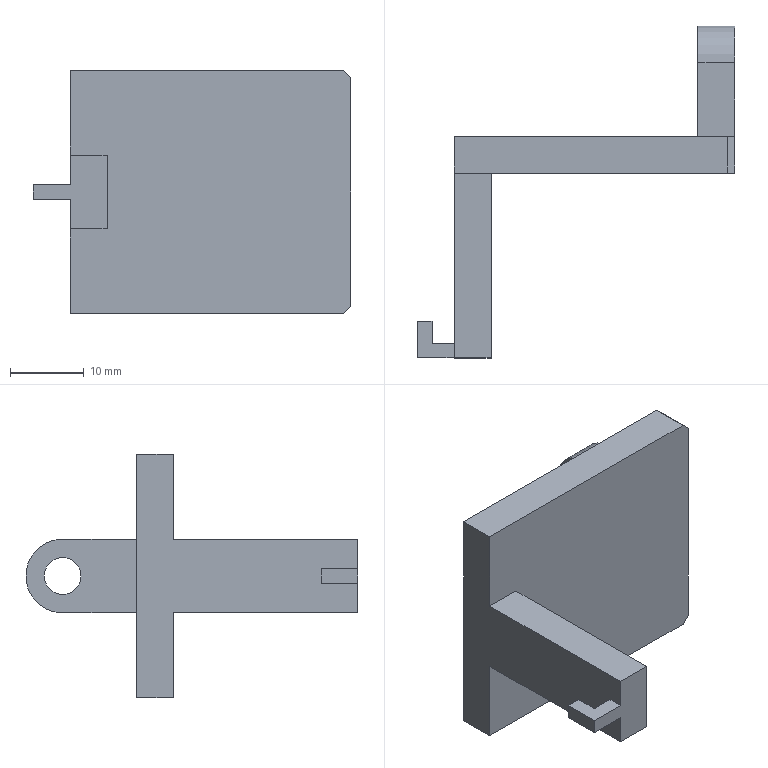Part | SolidWorks | 1 solid | 24 faces | box 43 x 45 x 33 mm | volume 8145 mm3 | plane 21 | cylinder 3 | commonest cylinder face diameters 5 x2 10 x1
STEP:
#1=CARTESIAN_POINT('',(30.5,25.,2.5));
#2=VERTEX_POINT('',#1);
#3=CARTESIAN_POINT('',(30.5,25.,-2.5));
#4=VERTEX_POINT('',#3);
#5=CARTESIAN_POINT('',(30.5,25.,0.));
#6=DIRECTION('',(1.,0.,0.));
#7=DIRECTION('',(0.,0.,-1.));
#8=AXIS2_PLACEMENT_3D('',#5,#6,#7);
#9=CIRCLE('',#8,2.5);
#10=EDGE_CURVE('',#2,#4,#9,.T.);
#11=ORIENTED_EDGE('',*,*,#10,.F.);
#12=CARTESIAN_POINT('',(35.5,25.,2.5));
#13=VERTEX_POINT('',#12);
#14=CARTESIAN_POINT('',(5.5,25.,2.5));
#15=DIRECTION('',(1.,0.,0.));
#16=VECTOR('',#15,1000.);
#17=LINE('',#14,#16);
#18=EDGE_CURVE('',#2,#13,#17,.T.);
#19=ORIENTED_EDGE('',*,*,#18,.T.);
#20=CARTESIAN_POINT('',(35.5,25.,-2.5));
#21=VERTEX_POINT('',#20);
#22=CARTESIAN_POINT('',(35.5,25.,0.));
#23=DIRECTION('',(1.,0.,0.));
#24=DIRECTION('',(0.,0.,-1.));
#25=AXIS2_PLACEMENT_3D('',#22,#23,#24);
#26=CIRCLE('',#25,2.5);
#27=EDGE_CURVE('',#13,#21,#26,.T.);
#28=ORIENTED_EDGE('',*,*,#27,.T.);
#29=CARTESIAN_POINT('',(5.5,25.,-2.5));
#30=DIRECTION('',(1.,0.,0.));
#31=VECTOR('',#30,1000.);
#32=LINE('',#29,#31);
#33=EDGE_CURVE('',#4,#21,#32,.T.);
#34=ORIENTED_EDGE('',*,*,#33,.F.);
#35=EDGE_LOOP('',(#11,#19,#28,#34));
#36=FACE_OUTER_BOUND('',#35,.T.);
#37=CARTESIAN_POINT('',(5.5,25.,0.));
#38=DIRECTION('',(1.,0.,0.));
#39=DIRECTION('',(0.,0.,-1.));
#40=AXIS2_PLACEMENT_3D('',#37,#38,#39);
#41=CYLINDRICAL_SURFACE('',#40,2.5);
#42=ADVANCED_FACE('',(#36),#41,.F.);
#43=CARTESIAN_POINT('',(-2.5,-13.,-1.));
#44=VERTEX_POINT('',#43);
#45=CARTESIAN_POINT('',(-2.5,-15.,-1.));
#46=VERTEX_POINT('',#45);
#47=CARTESIAN_POINT('',(-2.5,-15.,-1.));
#48=DIRECTION('',(0.,-1.,0.));
#49=VECTOR('',#48,1000.);
#50=LINE('',#47,#49);
#51=EDGE_CURVE('',#44,#46,#50,.T.);
#52=ORIENTED_EDGE('',*,*,#51,.F.);
#53=CARTESIAN_POINT('',(-2.5,-13.,1.));
#54=VERTEX_POINT('',#53);
#55=CARTESIAN_POINT('',(-2.5,-13.,1.));
#56=DIRECTION('',(0.,0.,-1.));
#57=VECTOR('',#56,1000.);
#58=LINE('',#55,#57);
#59=EDGE_CURVE('',#54,#44,#58,.T.);
#60=ORIENTED_EDGE('',*,*,#59,.F.);
#61=CARTESIAN_POINT('',(-2.5,-15.,1.));
#62=VERTEX_POINT('',#61);
#63=CARTESIAN_POINT('',(-2.5,-15.,1.));
#64=DIRECTION('',(0.,-1.,0.));
#65=VECTOR('',#64,1000.);
#66=LINE('',#63,#65);
#67=EDGE_CURVE('',#54,#62,#66,.T.);
#68=ORIENTED_EDGE('',*,*,#67,.T.);
#69=CARTESIAN_POINT('',(-2.5,-15.,5.));
#70=VERTEX_POINT('',#69);
#71=CARTESIAN_POINT('',(-2.5,-15.,16.5));
#72=DIRECTION('',(0.,0.,-1.));
#73=VECTOR('',#72,1000.);
#74=LINE('',#71,#73);
#75=EDGE_CURVE('',#70,#62,#74,.T.);
#76=ORIENTED_EDGE('',*,*,#75,.F.);
#77=CARTESIAN_POINT('',(-2.5,10.,5.));
#78=VERTEX_POINT('',#77);
#79=CARTESIAN_POINT('',(-2.5,0.,5.));
#80=DIRECTION('',(0.,1.,0.));
#81=VECTOR('',#80,1000.);
#82=LINE('',#79,#81);
#83=EDGE_CURVE('',#70,#78,#82,.T.);
#84=ORIENTED_EDGE('',*,*,#83,.T.);
#85=CARTESIAN_POINT('',(-2.5,10.,16.5));
#86=VERTEX_POINT('',#85);
#87=CARTESIAN_POINT('',(-2.5,10.,16.5));
#88=DIRECTION('',(0.,0.,1.));
#89=VECTOR('',#88,1000.);
#90=LINE('',#87,#89);
#91=EDGE_CURVE('',#78,#86,#90,.T.);
#92=ORIENTED_EDGE('',*,*,#91,.T.);
#93=CARTESIAN_POINT('',(-2.5,15.,16.5));
#94=VERTEX_POINT('',#93);
#95=CARTESIAN_POINT('',(-2.5,0.,16.5));
#96=DIRECTION('',(0.,-1.,0.));
#97=VECTOR('',#96,1000.);
#98=LINE('',#95,#97);
#99=EDGE_CURVE('',#94,#86,#98,.T.);
#100=ORIENTED_EDGE('',*,*,#99,.F.);
#101=CARTESIAN_POINT('',(-2.5,15.,-16.5));
#102=VERTEX_POINT('',#101);
#103=CARTESIAN_POINT('',(-2.5,15.,16.5));
#104=DIRECTION('',(0.,0.,-1.));
#105=VECTOR('',#104,1000.);
#106=LINE('',#103,#105);
#107=EDGE_CURVE('',#94,#102,#106,.T.);
#108=ORIENTED_EDGE('',*,*,#107,.T.);
#109=CARTESIAN_POINT('',(-2.5,10.,-16.5));
#110=VERTEX_POINT('',#109);
#111=CARTESIAN_POINT('',(-2.5,0.,-16.5));
#112=DIRECTION('',(0.,-1.,0.));
#113=VECTOR('',#112,1000.);
#114=LINE('',#111,#113);
#115=EDGE_CURVE('',#102,#110,#114,.T.);
#116=ORIENTED_EDGE('',*,*,#115,.T.);
#117=CARTESIAN_POINT('',(-2.5,10.,-5.));
#118=VERTEX_POINT('',#117);
#119=CARTESIAN_POINT('',(-2.5,10.,16.5));
#120=DIRECTION('',(0.,0.,1.));
#121=VECTOR('',#120,1000.);
#122=LINE('',#119,#121);
#123=EDGE_CURVE('',#110,#118,#122,.T.);
#124=ORIENTED_EDGE('',*,*,#123,.T.);
#125=CARTESIAN_POINT('',(-2.5,-15.,-5.));
#126=VERTEX_POINT('',#125);
#127=CARTESIAN_POINT('',(-2.5,0.,-5.));
#128=DIRECTION('',(0.,-1.,0.));
#129=VECTOR('',#128,1000.);
#130=LINE('',#127,#129);
#131=EDGE_CURVE('',#118,#126,#130,.T.);
#132=ORIENTED_EDGE('',*,*,#131,.T.);
#133=CARTESIAN_POINT('',(-2.5,-15.,16.5));
#134=DIRECTION('',(0.,0.,-1.));
#135=VECTOR('',#134,1000.);
#136=LINE('',#133,#135);
#137=EDGE_CURVE('',#46,#126,#136,.T.);
#138=ORIENTED_EDGE('',*,*,#137,.F.);
#139=EDGE_LOOP('',(#52,#60,#68,#76,#84,#92,#100,#108,#116,#124,#132,#138));
#140=FACE_OUTER_BOUND('',#139,.T.);
#141=CARTESIAN_POINT('',(-2.5,0.,16.5));
#142=DIRECTION('',(1.,0.,0.));
#143=DIRECTION('',(0.,1.,0.));
#144=AXIS2_PLACEMENT_3D('',#141,#142,#143);
#145=PLANE('',#144);
#146=ADVANCED_FACE('',(#140),#145,.F.);
#147=CARTESIAN_POINT('',(35.5,25.,0.));
#148=DIRECTION('',(1.,0.,0.));
#149=DIRECTION('',(0.,0.,-1.));
#150=AXIS2_PLACEMENT_3D('',#147,#148,#149);
#151=CIRCLE('',#150,2.5);
#152=EDGE_CURVE('',#21,#13,#151,.T.);
#153=ORIENTED_EDGE('',*,*,#152,.F.);
#154=ORIENTED_EDGE('',*,*,#27,.F.);
#155=EDGE_LOOP('',(#153,#154));
#156=FACE_BOUND('',#155,.T.);
#157=CARTESIAN_POINT('',(35.5,10.,15.5));
#158=VERTEX_POINT('',#157);
#159=CARTESIAN_POINT('',(35.5,10.,-15.5));
#160=VERTEX_POINT('',#159);
#161=CARTESIAN_POINT('',(35.5,10.,16.5));
#162=DIRECTION('',(0.,0.,-1.));
#163=VECTOR('',#162,1000.);
#164=LINE('',#161,#163);
#165=EDGE_CURVE('',#158,#160,#164,.T.);
#166=ORIENTED_EDGE('',*,*,#165,.T.);
#167=CARTESIAN_POINT('',(35.5,15.,-15.5));
#168=VERTEX_POINT('',#167);
#169=CARTESIAN_POINT('',(35.5,15.,-15.5));
#170=DIRECTION('',(0.,1.,0.));
#171=VECTOR('',#170,1000.);
#172=LINE('',#169,#171);
#173=EDGE_CURVE('',#160,#168,#172,.T.);
#174=ORIENTED_EDGE('',*,*,#173,.T.);
#175=CARTESIAN_POINT('',(35.5,15.,-5.));
#176=VERTEX_POINT('',#175);
#177=CARTESIAN_POINT('',(35.5,15.,16.5));
#178=DIRECTION('',(0.,0.,-1.));
#179=VECTOR('',#178,1000.);
#180=LINE('',#177,#179);
#181=EDGE_CURVE('',#176,#168,#180,.T.);
#182=ORIENTED_EDGE('',*,*,#181,.F.);
#183=CARTESIAN_POINT('',(35.5,25.,-5.));
#184=VERTEX_POINT('',#183);
#185=CARTESIAN_POINT('',(35.5,0.,-5.));
#186=DIRECTION('',(0.,1.,0.));
#187=VECTOR('',#186,1000.);
#188=LINE('',#185,#187);
#189=EDGE_CURVE('',#176,#184,#188,.T.);
#190=ORIENTED_EDGE('',*,*,#189,.T.);
#191=CARTESIAN_POINT('',(35.5,25.,5.));
#192=VERTEX_POINT('',#191);
#193=CARTESIAN_POINT('',(35.5,25.,0.));
#194=DIRECTION('',(1.,0.,0.));
#195=DIRECTION('',(0.,0.,-1.));
#196=AXIS2_PLACEMENT_3D('',#193,#194,#195);
#197=CIRCLE('',#196,5.);
#198=EDGE_CURVE('',#184,#192,#197,.T.);
#199=ORIENTED_EDGE('',*,*,#198,.T.);
#200=CARTESIAN_POINT('',(35.5,15.,5.));
#201=VERTEX_POINT('',#200);
#202=CARTESIAN_POINT('',(35.5,0.,5.));
#203=DIRECTION('',(0.,1.,0.));
#204=VECTOR('',#203,1000.);
#205=LINE('',#202,#204);
#206=EDGE_CURVE('',#201,#192,#205,.T.);
#207=ORIENTED_EDGE('',*,*,#206,.F.);
#208=CARTESIAN_POINT('',(35.5,15.,15.5));
#209=VERTEX_POINT('',#208);
#210=CARTESIAN_POINT('',(35.5,15.,16.5));
#211=DIRECTION('',(0.,0.,-1.));
#212=VECTOR('',#211,1000.);
#213=LINE('',#210,#212);
#214=EDGE_CURVE('',#209,#201,#213,.T.);
#215=ORIENTED_EDGE('',*,*,#214,.F.);
#216=CARTESIAN_POINT('',(35.5,0.,15.5));
#217=DIRECTION('',(0.,-1.,0.));
#218=VECTOR('',#217,1000.);
#219=LINE('',#216,#218);
#220=EDGE_CURVE('',#209,#158,#219,.T.);
#221=ORIENTED_EDGE('',*,*,#220,.T.);
#222=EDGE_LOOP('',(#166,#174,#182,#190,#199,#207,#215,#221));
#223=FACE_OUTER_BOUND('',#222,.T.);
#224=CARTESIAN_POINT('',(35.5,0.,16.5));
#225=DIRECTION('',(1.,0.,0.));
#226=DIRECTION('',(0.,1.,0.));
#227=AXIS2_PLACEMENT_3D('',#224,#225,#226);
#228=PLANE('',#227);
#229=ADVANCED_FACE('',(#156,#223),#228,.T.);
#230=ORIENTED_EDGE('',*,*,#181,.T.);
#231=CARTESIAN_POINT('',(34.5,15.,-16.5));
#232=VERTEX_POINT('',#231);
#233=CARTESIAN_POINT('',(33.75,15.,-17.25));
#234=DIRECTION('',(-0.7071,0.,-0.7071));
#235=VECTOR('',#234,1000.);
#236=LINE('',#233,#235);
#237=EDGE_CURVE('',#168,#232,#236,.T.);
#238=ORIENTED_EDGE('',*,*,#237,.T.);
#239=CARTESIAN_POINT('',(0.,15.,-16.5));
#240=DIRECTION('',(1.,0.,0.));
#241=VECTOR('',#240,1000.);
#242=LINE('',#239,#241);
#243=EDGE_CURVE('',#102,#232,#242,.T.);
#244=ORIENTED_EDGE('',*,*,#243,.F.);
#245=ORIENTED_EDGE('',*,*,#107,.F.);
#246=CARTESIAN_POINT('',(34.5,15.,16.5));
#247=VERTEX_POINT('',#246);
#248=CARTESIAN_POINT('',(0.,15.,16.5));
#249=DIRECTION('',(1.,0.,0.));
#250=VECTOR('',#249,1000.);
#251=LINE('',#248,#250);
#252=EDGE_CURVE('',#94,#247,#251,.T.);
#253=ORIENTED_EDGE('',*,*,#252,.T.);
#254=CARTESIAN_POINT('',(17.25,15.,33.75));
#255=DIRECTION('',(0.7071,0.,-0.7071));
#256=VECTOR('',#255,1000.);
#257=LINE('',#254,#256);
#258=EDGE_CURVE('',#247,#209,#257,.T.);
#259=ORIENTED_EDGE('',*,*,#258,.T.);
#260=ORIENTED_EDGE('',*,*,#214,.T.);
#261=CARTESIAN_POINT('',(30.5,15.,5.));
#262=VERTEX_POINT('',#261);
#263=CARTESIAN_POINT('',(30.5,15.,5.));
#264=DIRECTION('',(1.,0.,0.));
#265=VECTOR('',#264,1000.);
#266=LINE('',#263,#265);
#267=EDGE_CURVE('',#262,#201,#266,.T.);
#268=ORIENTED_EDGE('',*,*,#267,.F.);
#269=CARTESIAN_POINT('',(30.5,15.,-5.));
#270=VERTEX_POINT('',#269);
#271=CARTESIAN_POINT('',(30.5,15.,0.));
#272=DIRECTION('',(0.,0.,1.));
#273=VECTOR('',#272,1000.);
#274=LINE('',#271,#273);
#275=EDGE_CURVE('',#270,#262,#274,.T.);
#276=ORIENTED_EDGE('',*,*,#275,.F.);
#277=CARTESIAN_POINT('',(30.5,15.,-5.));
#278=DIRECTION('',(1.,0.,0.));
#279=VECTOR('',#278,1000.);
#280=LINE('',#277,#279);
#281=EDGE_CURVE('',#270,#176,#280,.T.);
#282=ORIENTED_EDGE('',*,*,#281,.T.);
#283=EDGE_LOOP('',(#230,#238,#244,#245,#253,#259,#260,#268,#276,#282));
#284=FACE_OUTER_BOUND('',#283,.T.);
#285=CARTESIAN_POINT('',(0.,15.,16.5));
#286=DIRECTION('',(0.,1.,0.));
#287=DIRECTION('',(0.,0.,1.));
#288=AXIS2_PLACEMENT_3D('',#285,#286,#287);
#289=PLANE('',#288);
#290=ADVANCED_FACE('',(#284),#289,.T.);
#291=CARTESIAN_POINT('',(2.5,-15.,5.));
#292=VERTEX_POINT('',#291);
#293=CARTESIAN_POINT('',(2.5,-15.,-5.));
#294=VERTEX_POINT('',#293);
#295=CARTESIAN_POINT('',(2.5,-15.,16.5));
#296=DIRECTION('',(0.,0.,-1.));
#297=VECTOR('',#296,1000.);
#298=LINE('',#295,#297);
#299=EDGE_CURVE('',#292,#294,#298,.T.);
#300=ORIENTED_EDGE('',*,*,#299,.F.);
#301=CARTESIAN_POINT('',(-12.5,-15.,5.));
#302=DIRECTION('',(1.,0.,0.));
#303=VECTOR('',#302,1000.);
#304=LINE('',#301,#303);
#305=EDGE_CURVE('',#70,#292,#304,.T.);
#306=ORIENTED_EDGE('',*,*,#305,.F.);
#307=ORIENTED_EDGE('',*,*,#75,.T.);
#308=CARTESIAN_POINT('',(-7.5,-15.,1.));
#309=VERTEX_POINT('',#308);
#310=CARTESIAN_POINT('',(-2.5,-15.,1.));
#311=DIRECTION('',(-1.,0.,0.));
#312=VECTOR('',#311,1000.);
#313=LINE('',#310,#312);
#314=EDGE_CURVE('',#62,#309,#313,.T.);
#315=ORIENTED_EDGE('',*,*,#314,.T.);
#316=CARTESIAN_POINT('',(-7.5,-15.,-1.));
#317=VERTEX_POINT('',#316);
#318=CARTESIAN_POINT('',(-7.5,-15.,1.));
#319=DIRECTION('',(0.,0.,-1.));
#320=VECTOR('',#319,1000.);
#321=LINE('',#318,#320);
#322=EDGE_CURVE('',#309,#317,#321,.T.);
#323=ORIENTED_EDGE('',*,*,#322,.T.);
#324=CARTESIAN_POINT('',(-2.5,-15.,-1.));
#325=DIRECTION('',(-1.,0.,0.));
#326=VECTOR('',#325,1000.);
#327=LINE('',#324,#326);
#328=EDGE_CURVE('',#46,#317,#327,.T.);
#329=ORIENTED_EDGE('',*,*,#328,.F.);
#330=ORIENTED_EDGE('',*,*,#137,.T.);
#331=CARTESIAN_POINT('',(-12.5,-15.,-5.));
#332=DIRECTION('',(1.,0.,0.));
#333=VECTOR('',#332,1000.);
#334=LINE('',#331,#333);
#335=EDGE_CURVE('',#126,#294,#334,.T.);
#336=ORIENTED_EDGE('',*,*,#335,.T.);
#337=EDGE_LOOP('',(#300,#306,#307,#315,#323,#329,#330,#336));
#338=FACE_OUTER_BOUND('',#337,.T.);
#339=CARTESIAN_POINT('',(0.,-15.,16.5));
#340=DIRECTION('',(0.,1.,0.));
#341=DIRECTION('',(0.,0.,1.));
#342=AXIS2_PLACEMENT_3D('',#339,#340,#341);
#343=PLANE('',#342);
#344=ADVANCED_FACE('',(#338),#343,.F.);
#345=CARTESIAN_POINT('',(2.5,10.,5.));
#346=VERTEX_POINT('',#345);
#347=CARTESIAN_POINT('',(2.5,0.,5.));
#348=DIRECTION('',(0.,1.,0.));
#349=VECTOR('',#348,1000.);
#350=LINE('',#347,#349);
#351=EDGE_CURVE('',#292,#346,#350,.T.);
#352=ORIENTED_EDGE('',*,*,#351,.F.);
#353=ORIENTED_EDGE('',*,*,#299,.T.);
#354=CARTESIAN_POINT('',(2.5,10.,-5.));
#355=VERTEX_POINT('',#354);
#356=CARTESIAN_POINT('',(2.5,0.,-5.));
#357=DIRECTION('',(0.,-1.,0.));
#358=VECTOR('',#357,1000.);
#359=LINE('',#356,#358);
#360=EDGE_CURVE('',#355,#294,#359,.T.);
#361=ORIENTED_EDGE('',*,*,#360,.F.);
#362=CARTESIAN_POINT('',(2.5,10.,16.5));
#363=DIRECTION('',(0.,0.,-1.));
#364=VECTOR('',#363,1000.);
#365=LINE('',#362,#364);
#366=EDGE_CURVE('',#346,#355,#365,.T.);
#367=ORIENTED_EDGE('',*,*,#366,.F.);
#368=EDGE_LOOP('',(#352,#353,#361,#367));
#369=FACE_OUTER_BOUND('',#368,.T.);
#370=CARTESIAN_POINT('',(2.5,0.,16.5));
#371=DIRECTION('',(1.,0.,0.));
#372=DIRECTION('',(0.,1.,0.));
#373=AXIS2_PLACEMENT_3D('',#370,#371,#372);
#374=PLANE('',#373);
#375=ADVANCED_FACE('',(#369),#374,.T.);
#376=CARTESIAN_POINT('',(34.5,10.,16.5));
#377=VERTEX_POINT('',#376);
#378=CARTESIAN_POINT('',(0.,10.,16.5));
#379=DIRECTION('',(1.,0.,0.));
#380=VECTOR('',#379,1000.);
#381=LINE('',#378,#380);
#382=EDGE_CURVE('',#86,#377,#381,.T.);
#383=ORIENTED_EDGE('',*,*,#382,.F.);
#384=ORIENTED_EDGE('',*,*,#91,.F.);
#385=CARTESIAN_POINT('',(-12.5,10.,5.));
#386=DIRECTION('',(1.,0.,0.));
#387=VECTOR('',#386,1000.);
#388=LINE('',#385,#387);
#389=EDGE_CURVE('',#78,#346,#388,.T.);
#390=ORIENTED_EDGE('',*,*,#389,.T.);
#391=ORIENTED_EDGE('',*,*,#366,.T.);
#392=CARTESIAN_POINT('',(-12.5,10.,-5.));
#393=DIRECTION('',(1.,0.,0.));
#394=VECTOR('',#393,1000.);
#395=LINE('',#392,#394);
#396=EDGE_CURVE('',#118,#355,#395,.T.);
#397=ORIENTED_EDGE('',*,*,#396,.F.);
#398=ORIENTED_EDGE('',*,*,#123,.F.);
#399=CARTESIAN_POINT('',(34.5,10.,-16.5));
#400=VERTEX_POINT('',#399);
#401=CARTESIAN_POINT('',(0.,10.,-16.5));
#402=DIRECTION('',(1.,0.,0.));
#403=VECTOR('',#402,1000.);
#404=LINE('',#401,#403);
#405=EDGE_CURVE('',#110,#400,#404,.T.);
#406=ORIENTED_EDGE('',*,*,#405,.T.);
#407=CARTESIAN_POINT('',(34.5,10.,-16.5));
#408=DIRECTION('',(0.7071,0.,0.7071));
#409=VECTOR('',#408,1000.);
#410=LINE('',#407,#409);
#411=EDGE_CURVE('',#400,#160,#410,.T.);
#412=ORIENTED_EDGE('',*,*,#411,.T.);
#413=ORIENTED_EDGE('',*,*,#165,.F.);
#414=CARTESIAN_POINT('',(35.5,10.,15.5));
#415=DIRECTION('',(-0.7071,0.,0.7071));
#416=VECTOR('',#415,1000.);
#417=LINE('',#414,#416);
#418=EDGE_CURVE('',#158,#377,#417,.T.);
#419=ORIENTED_EDGE('',*,*,#418,.T.);
#420=EDGE_LOOP('',(#383,#384,#390,#391,#397,#398,#406,#412,#413,#419));
#421=FACE_OUTER_BOUND('',#420,.T.);
#422=CARTESIAN_POINT('',(0.,10.,16.5));
#423=DIRECTION('',(0.,1.,0.));
#424=DIRECTION('',(0.,0.,1.));
#425=AXIS2_PLACEMENT_3D('',#422,#423,#424);
#426=PLANE('',#425);
#427=ADVANCED_FACE('',(#421),#426,.F.);
#428=ORIENTED_EDGE('',*,*,#99,.T.);
#429=ORIENTED_EDGE('',*,*,#382,.T.);
#430=CARTESIAN_POINT('',(34.5,0.,16.5));
#431=DIRECTION('',(0.,1.,0.));
#432=VECTOR('',#431,1000.);
#433=LINE('',#430,#432);
#434=EDGE_CURVE('',#377,#247,#433,.T.);
#435=ORIENTED_EDGE('',*,*,#434,.T.);
#436=ORIENTED_EDGE('',*,*,#252,.F.);
#437=EDGE_LOOP('',(#428,#429,#435,#436));
#438=FACE_OUTER_BOUND('',#437,.T.);
#439=CARTESIAN_POINT('',(0.,0.,16.5));
#440=DIRECTION('',(0.,0.,1.));
#441=DIRECTION('',(1.,0.,0.));
#442=AXIS2_PLACEMENT_3D('',#439,#440,#441);
#443=PLANE('',#442);
#444=ADVANCED_FACE('',(#438),#443,.T.);
#445=ORIENTED_EDGE('',*,*,#405,.F.);
#446=ORIENTED_EDGE('',*,*,#115,.F.);
#447=ORIENTED_EDGE('',*,*,#243,.T.);
#448=CARTESIAN_POINT('',(34.5,10.,-16.5));
#449=DIRECTION('',(0.,-1.,0.));
#450=VECTOR('',#449,1000.);
#451=LINE('',#448,#450);
#452=EDGE_CURVE('',#232,#400,#451,.T.);
#453=ORIENTED_EDGE('',*,*,#452,.T.);
#454=EDGE_LOOP('',(#445,#446,#447,#453));
#455=FACE_OUTER_BOUND('',#454,.T.);
#456=CARTESIAN_POINT('',(0.,0.,-16.5));
#457=DIRECTION('',(0.,0.,1.));
#458=DIRECTION('',(1.,0.,0.));
#459=AXIS2_PLACEMENT_3D('',#456,#457,#458);
#460=PLANE('',#459);
#461=ADVANCED_FACE('',(#455),#460,.F.);
#462=ORIENTED_EDGE('',*,*,#189,.F.);
#463=ORIENTED_EDGE('',*,*,#281,.F.);
#464=CARTESIAN_POINT('',(30.5,25.,-5.));
#465=VERTEX_POINT('',#464);
#466=CARTESIAN_POINT('',(30.5,0.,-5.));
#467=DIRECTION('',(0.,1.,0.));
#468=VECTOR('',#467,1000.);
#469=LINE('',#466,#468);
#470=EDGE_CURVE('',#270,#465,#469,.T.);
#471=ORIENTED_EDGE('',*,*,#470,.T.);
#472=CARTESIAN_POINT('',(30.5,25.,-5.));
#473=DIRECTION('',(1.,0.,0.));
#474=VECTOR('',#473,1000.);
#475=LINE('',#472,#474);
#476=EDGE_CURVE('',#465,#184,#475,.T.);
#477=ORIENTED_EDGE('',*,*,#476,.T.);
#478=EDGE_LOOP('',(#462,#463,#471,#477));
#479=FACE_OUTER_BOUND('',#478,.T.);
#480=CARTESIAN_POINT('',(30.5,0.,-5.));
#481=DIRECTION('',(0.,0.,-1.));
#482=DIRECTION('',(0.,1.,0.));
#483=AXIS2_PLACEMENT_3D('',#480,#481,#482);
#484=PLANE('',#483);
#485=ADVANCED_FACE('',(#479),#484,.T.);
#486=ORIENTED_EDGE('',*,*,#206,.T.);
#487=CARTESIAN_POINT('',(30.5,25.,5.));
#488=VERTEX_POINT('',#487);
#489=CARTESIAN_POINT('',(30.5,25.,5.));
#490=DIRECTION('',(1.,0.,0.));
#491=VECTOR('',#490,1000.);
#492=LINE('',#489,#491);
#493=EDGE_CURVE('',#488,#192,#492,.T.);
#494=ORIENTED_EDGE('',*,*,#493,.F.);
#495=CARTESIAN_POINT('',(30.5,0.,5.));
#496=DIRECTION('',(0.,1.,0.));
#497=VECTOR('',#496,1000.);
#498=LINE('',#495,#497);
#499=EDGE_CURVE('',#262,#488,#498,.T.);
#500=ORIENTED_EDGE('',*,*,#499,.F.);
#501=ORIENTED_EDGE('',*,*,#267,.T.);
#502=EDGE_LOOP('',(#486,#494,#500,#501));
#503=FACE_OUTER_BOUND('',#502,.T.);
#504=CARTESIAN_POINT('',(30.5,0.,5.));
#505=DIRECTION('',(0.,0.,-1.));
#506=DIRECTION('',(0.,1.,0.));
#507=AXIS2_PLACEMENT_3D('',#504,#505,#506);
#508=PLANE('',#507);
#509=ADVANCED_FACE('',(#503),#508,.F.);
#510=ORIENTED_EDGE('',*,*,#198,.F.);
#511=ORIENTED_EDGE('',*,*,#476,.F.);
#512=CARTESIAN_POINT('',(30.5,25.,0.));
#513=DIRECTION('',(1.,0.,0.));
#514=DIRECTION('',(0.,0.,-1.));
#515=AXIS2_PLACEMENT_3D('',#512,#513,#514);
#516=CIRCLE('',#515,5.);
#517=EDGE_CURVE('',#465,#488,#516,.T.);
#518=ORIENTED_EDGE('',*,*,#517,.T.);
#519=ORIENTED_EDGE('',*,*,#493,.T.);
#520=EDGE_LOOP('',(#510,#511,#518,#519));
#521=FACE_OUTER_BOUND('',#520,.T.);
#522=CARTESIAN_POINT('',(30.5,25.,0.));
#523=DIRECTION('',(1.,0.,0.));
#524=DIRECTION('',(0.,0.,-1.));
#525=AXIS2_PLACEMENT_3D('',#522,#523,#524);
#526=CYLINDRICAL_SURFACE('',#525,5.);
#527=ADVANCED_FACE('',(#521),#526,.T.);
#528=CARTESIAN_POINT('',(30.5,25.,0.));
#529=DIRECTION('',(1.,0.,0.));
#530=DIRECTION('',(0.,0.,-1.));
#531=AXIS2_PLACEMENT_3D('',#528,#529,#530);
#532=CIRCLE('',#531,2.5);
#533=EDGE_CURVE('',#4,#2,#532,.T.);
#534=ORIENTED_EDGE('',*,*,#533,.T.);
#535=ORIENTED_EDGE('',*,*,#10,.T.);
#536=EDGE_LOOP('',(#534,#535));
#537=FACE_BOUND('',#536,.T.);
#538=ORIENTED_EDGE('',*,*,#470,.F.);
#539=ORIENTED_EDGE('',*,*,#275,.T.);
#540=ORIENTED_EDGE('',*,*,#499,.T.);
#541=ORIENTED_EDGE('',*,*,#517,.F.);
#542=EDGE_LOOP('',(#538,#539,#540,#541));
#543=FACE_OUTER_BOUND('',#542,.T.);
#544=CARTESIAN_POINT('',(30.5,0.,0.));
#545=DIRECTION('',(1.,0.,0.));
#546=DIRECTION('',(0.,0.,-1.));
#547=AXIS2_PLACEMENT_3D('',#544,#545,#546);
#548=PLANE('',#547);
#549=ADVANCED_FACE('',(#537,#543),#548,.F.);
#550=ORIENTED_EDGE('',*,*,#237,.F.);
#551=ORIENTED_EDGE('',*,*,#173,.F.);
#552=ORIENTED_EDGE('',*,*,#411,.F.);
#553=ORIENTED_EDGE('',*,*,#452,.F.);
#554=EDGE_LOOP('',(#550,#551,#552,#553));
#555=FACE_OUTER_BOUND('',#554,.T.);
#556=CARTESIAN_POINT('',(34.5,0.,-16.5));
#557=DIRECTION('',(0.7071,0.,-0.7071));
#558=DIRECTION('',(0.,1.,0.));
#559=AXIS2_PLACEMENT_3D('',#556,#557,#558);
#560=PLANE('',#559);
#561=ADVANCED_FACE('',(#555),#560,.T.);
#562=ORIENTED_EDGE('',*,*,#258,.F.);
#563=ORIENTED_EDGE('',*,*,#434,.F.);
#564=ORIENTED_EDGE('',*,*,#418,.F.);
#565=ORIENTED_EDGE('',*,*,#220,.F.);
#566=EDGE_LOOP('',(#562,#563,#564,#565));
#567=FACE_OUTER_BOUND('',#566,.T.);
#568=CARTESIAN_POINT('',(35.5,0.,15.5));
#569=DIRECTION('',(-0.7071,0.,-0.7071));
#570=DIRECTION('',(0.,-1.,0.));
#571=AXIS2_PLACEMENT_3D('',#568,#569,#570);
#572=PLANE('',#571);
#573=ADVANCED_FACE('',(#567),#572,.F.);
#574=ORIENTED_EDGE('',*,*,#18,.F.);
#575=ORIENTED_EDGE('',*,*,#533,.F.);
#576=ORIENTED_EDGE('',*,*,#33,.T.);
#577=ORIENTED_EDGE('',*,*,#152,.T.);
#578=EDGE_LOOP('',(#574,#575,#576,#577));
#579=FACE_OUTER_BOUND('',#578,.T.);
#580=CARTESIAN_POINT('',(5.5,25.,0.));
#581=DIRECTION('',(1.,0.,0.));
#582=DIRECTION('',(0.,0.,-1.));
#583=AXIS2_PLACEMENT_3D('',#580,#581,#582);
#584=CYLINDRICAL_SURFACE('',#583,2.5);
#585=ADVANCED_FACE('',(#579),#584,.F.);
#586=ORIENTED_EDGE('',*,*,#396,.T.);
#587=ORIENTED_EDGE('',*,*,#360,.T.);
#588=ORIENTED_EDGE('',*,*,#335,.F.);
#589=ORIENTED_EDGE('',*,*,#131,.F.);
#590=EDGE_LOOP('',(#586,#587,#588,#589));
#591=FACE_OUTER_BOUND('',#590,.T.);
#592=CARTESIAN_POINT('',(-12.5,10.,-5.));
#593=DIRECTION('',(0.,0.,1.));
#594=DIRECTION('',(0.,-1.,0.));
#595=AXIS2_PLACEMENT_3D('',#592,#593,#594);
#596=PLANE('',#595);
#597=ADVANCED_FACE('',(#591),#596,.F.);
#598=ORIENTED_EDGE('',*,*,#305,.T.);
#599=ORIENTED_EDGE('',*,*,#351,.T.);
#600=ORIENTED_EDGE('',*,*,#389,.F.);
#601=ORIENTED_EDGE('',*,*,#83,.F.);
#602=EDGE_LOOP('',(#598,#599,#600,#601));
#603=FACE_OUTER_BOUND('',#602,.T.);
#604=CARTESIAN_POINT('',(-12.5,10.,5.));
#605=DIRECTION('',(0.,0.,-1.));
#606=DIRECTION('',(0.,1.,0.));
#607=AXIS2_PLACEMENT_3D('',#604,#605,#606);
#608=PLANE('',#607);
#609=ADVANCED_FACE('',(#603),#608,.F.);
#610=CARTESIAN_POINT('',(-5.5,-13.,-1.));
#611=VERTEX_POINT('',#610);
#612=CARTESIAN_POINT('',(-2.5,-13.,-1.));
#613=DIRECTION('',(1.,0.,0.));
#614=VECTOR('',#613,1000.);
#615=LINE('',#612,#614);
#616=EDGE_CURVE('',#611,#44,#615,.T.);
#617=ORIENTED_EDGE('',*,*,#616,.F.);
#618=CARTESIAN_POINT('',(-5.5,-13.,1.));
#619=VERTEX_POINT('',#618);
#620=CARTESIAN_POINT('',(-5.5,-13.,1.));
#621=DIRECTION('',(0.,0.,-1.));
#622=VECTOR('',#621,1000.);
#623=LINE('',#620,#622);
#624=EDGE_CURVE('',#619,#611,#623,.T.);
#625=ORIENTED_EDGE('',*,*,#624,.F.);
#626=CARTESIAN_POINT('',(-2.5,-13.,1.));
#627=DIRECTION('',(1.,0.,0.));
#628=VECTOR('',#627,1000.);
#629=LINE('',#626,#628);
#630=EDGE_CURVE('',#619,#54,#629,.T.);
#631=ORIENTED_EDGE('',*,*,#630,.T.);
#632=ORIENTED_EDGE('',*,*,#59,.T.);
#633=EDGE_LOOP('',(#617,#625,#631,#632));
#634=FACE_OUTER_BOUND('',#633,.T.);
#635=CARTESIAN_POINT('',(-2.5,-13.,1.));
#636=DIRECTION('',(0.,1.,0.));
#637=DIRECTION('',(0.,0.,1.));
#638=AXIS2_PLACEMENT_3D('',#635,#636,#637);
#639=PLANE('',#638);
#640=ADVANCED_FACE('',(#634),#639,.T.);
#641=CARTESIAN_POINT('',(-5.5,-10.,-1.));
#642=VERTEX_POINT('',#641);
#643=CARTESIAN_POINT('',(-5.5,-13.,-1.));
#644=DIRECTION('',(0.,-1.,0.));
#645=VECTOR('',#644,1000.);
#646=LINE('',#643,#645);
#647=EDGE_CURVE('',#642,#611,#646,.T.);
#648=ORIENTED_EDGE('',*,*,#647,.F.);
#649=CARTESIAN_POINT('',(-5.5,-10.,1.));
#650=VERTEX_POINT('',#649);
#651=CARTESIAN_POINT('',(-5.5,-10.,1.));
#652=DIRECTION('',(0.,0.,-1.));
#653=VECTOR('',#652,1000.);
#654=LINE('',#651,#653);
#655=EDGE_CURVE('',#650,#642,#654,.T.);
#656=ORIENTED_EDGE('',*,*,#655,.F.);
#657=CARTESIAN_POINT('',(-5.5,-13.,1.));
#658=DIRECTION('',(0.,-1.,0.));
#659=VECTOR('',#658,1000.);
#660=LINE('',#657,#659);
#661=EDGE_CURVE('',#650,#619,#660,.T.);
#662=ORIENTED_EDGE('',*,*,#661,.T.);
#663=ORIENTED_EDGE('',*,*,#624,.T.);
#664=EDGE_LOOP('',(#648,#656,#662,#663));
#665=FACE_OUTER_BOUND('',#664,.T.);
#666=CARTESIAN_POINT('',(-5.5,-13.,1.));
#667=DIRECTION('',(1.,0.,0.));
#668=DIRECTION('',(0.,0.,-1.));
#669=AXIS2_PLACEMENT_3D('',#666,#667,#668);
#670=PLANE('',#669);
#671=ADVANCED_FACE('',(#665),#670,.T.);
#672=CARTESIAN_POINT('',(-7.5,-10.,-1.));
#673=VERTEX_POINT('',#672);
#674=CARTESIAN_POINT('',(-7.5,-10.,-1.));
#675=DIRECTION('',(1.,0.,0.));
#676=VECTOR('',#675,1000.);
#677=LINE('',#674,#676);
#678=EDGE_CURVE('',#673,#642,#677,.T.);
#679=ORIENTED_EDGE('',*,*,#678,.F.);
#680=CARTESIAN_POINT('',(-7.5,-10.,1.));
#681=VERTEX_POINT('',#680);
#682=CARTESIAN_POINT('',(-7.5,-10.,1.));
#683=DIRECTION('',(0.,0.,-1.));
#684=VECTOR('',#683,1000.);
#685=LINE('',#682,#684);
#686=EDGE_CURVE('',#681,#673,#685,.T.);
#687=ORIENTED_EDGE('',*,*,#686,.F.);
#688=CARTESIAN_POINT('',(-7.5,-10.,1.));
#689=DIRECTION('',(1.,0.,0.));
#690=VECTOR('',#689,1000.);
#691=LINE('',#688,#690);
#692=EDGE_CURVE('',#681,#650,#691,.T.);
#693=ORIENTED_EDGE('',*,*,#692,.T.);
#694=ORIENTED_EDGE('',*,*,#655,.T.);
#695=EDGE_LOOP('',(#679,#687,#693,#694));
#696=FACE_OUTER_BOUND('',#695,.T.);
#697=CARTESIAN_POINT('',(-7.5,-10.,1.));
#698=DIRECTION('',(0.,1.,0.));
#699=DIRECTION('',(0.,0.,1.));
#700=AXIS2_PLACEMENT_3D('',#697,#698,#699);
#701=PLANE('',#700);
#702=ADVANCED_FACE('',(#696),#701,.T.);
#703=CARTESIAN_POINT('',(-7.5,-15.,-1.));
#704=DIRECTION('',(0.,1.,0.));
#705=VECTOR('',#704,1000.);
#706=LINE('',#703,#705);
#707=EDGE_CURVE('',#317,#673,#706,.T.);
#708=ORIENTED_EDGE('',*,*,#707,.F.);
#709=ORIENTED_EDGE('',*,*,#322,.F.);
#710=CARTESIAN_POINT('',(-7.5,-15.,1.));
#711=DIRECTION('',(0.,1.,0.));
#712=VECTOR('',#711,1000.);
#713=LINE('',#710,#712);
#714=EDGE_CURVE('',#309,#681,#713,.T.);
#715=ORIENTED_EDGE('',*,*,#714,.T.);
#716=ORIENTED_EDGE('',*,*,#686,.T.);
#717=EDGE_LOOP('',(#708,#709,#715,#716));
#718=FACE_OUTER_BOUND('',#717,.T.);
#719=CARTESIAN_POINT('',(-7.5,-15.,1.));
#720=DIRECTION('',(-1.,0.,0.));
#721=DIRECTION('',(0.,0.,1.));
#722=AXIS2_PLACEMENT_3D('',#719,#720,#721);
#723=PLANE('',#722);
#724=ADVANCED_FACE('',(#718),#723,.T.);
#725=ORIENTED_EDGE('',*,*,#67,.F.);
#726=ORIENTED_EDGE('',*,*,#630,.F.);
#727=ORIENTED_EDGE('',*,*,#661,.F.);
#728=ORIENTED_EDGE('',*,*,#692,.F.);
#729=ORIENTED_EDGE('',*,*,#714,.F.);
#730=ORIENTED_EDGE('',*,*,#314,.F.);
#731=EDGE_LOOP('',(#725,#726,#727,#728,#729,#730));
#732=FACE_OUTER_BOUND('',#731,.T.);
#733=CARTESIAN_POINT('',(0.,0.,1.));
#734=DIRECTION('',(0.,0.,1.));
#735=DIRECTION('',(1.,0.,0.));
#736=AXIS2_PLACEMENT_3D('',#733,#734,#735);
#737=PLANE('',#736);
#738=ADVANCED_FACE('',(#732),#737,.T.);
#739=ORIENTED_EDGE('',*,*,#51,.T.);
#740=ORIENTED_EDGE('',*,*,#328,.T.);
#741=ORIENTED_EDGE('',*,*,#707,.T.);
#742=ORIENTED_EDGE('',*,*,#678,.T.);
#743=ORIENTED_EDGE('',*,*,#647,.T.);
#744=ORIENTED_EDGE('',*,*,#616,.T.);
#745=EDGE_LOOP('',(#739,#740,#741,#742,#743,#744));
#746=FACE_OUTER_BOUND('',#745,.T.);
#747=CARTESIAN_POINT('',(0.,0.,-1.));
#748=DIRECTION('',(0.,0.,1.));
#749=DIRECTION('',(1.,0.,0.));
#750=AXIS2_PLACEMENT_3D('',#747,#748,#749);
#751=PLANE('',#750);
#752=ADVANCED_FACE('',(#746),#751,.F.);
#753=CLOSED_SHELL('',(#42,#146,#229,#290,#344,#375,#427,#444,#461,#485,#509,#527,#549,#561,#573,#585,#597,#609,#640,#671,#702,#724,#738,#752));
#754=MANIFOLD_SOLID_BREP('',#753);
#755=CARTESIAN_POINT('',(0.,0.,0.));
#756=DIRECTION('',(0.,0.,1.));
#757=DIRECTION('',(1.,0.,0.));
#758=AXIS2_PLACEMENT_3D('',#755,#756,#757);
#759=(LENGTH_UNIT()NAMED_UNIT(*)SI_UNIT(.MILLI.,.METRE.));
#760=UNCERTAINTY_MEASURE_WITH_UNIT(LENGTH_MEASURE(0.00001),#759,'','');
#761=(NAMED_UNIT(*)PLANE_ANGLE_UNIT()SI_UNIT($,.RADIAN.));
#762=(NAMED_UNIT(*)SI_UNIT($,.STERADIAN.)SOLID_ANGLE_UNIT());
#763=(GEOMETRIC_REPRESENTATION_CONTEXT(3)GLOBAL_UNCERTAINTY_ASSIGNED_CONTEXT((#760))GLOBAL_UNIT_ASSIGNED_CONTEXT((#759,#761,#762))REPRESENTATION_CONTEXT('',''));
#764=ADVANCED_BREP_SHAPE_REPRESENTATION('',(#754,#758),#763);